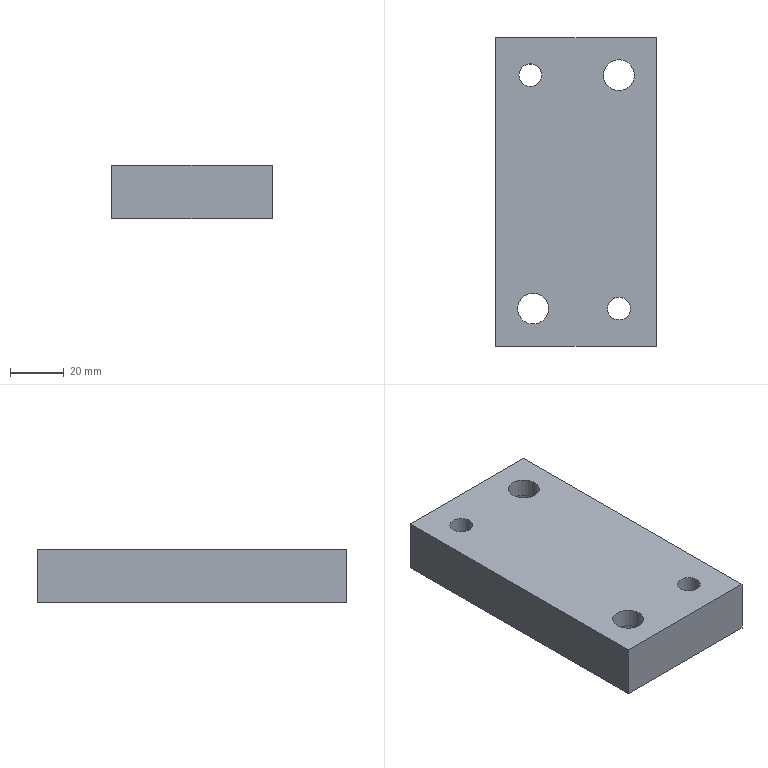Part | STEP file | lll_id610_x_t | 1 solid | 14 faces | box 60 x 115 x 20 mm | volume 127650 mm3 | plane 8 | cylinder 6 | commonest cylinder face diameters 8.505 x2 11.509 x2 18.007 x2
STEP:
#1=CARTESIAN_POINT('',(1834.747,-196.,132.5));
#2=VERTEX_POINT('',#1);
#3=CARTESIAN_POINT('',(1839.,-196.,132.5));
#4=DIRECTION('',(0.,0.,-1.));
#5=DIRECTION('',(-1.,0.,0.));
#6=AXIS2_PLACEMENT_3D('',#3,#4,#5);
#7=CIRCLE('',#6,4.253);
#8=EDGE_CURVE('',#2,#2,#7,.T.);
#9=ORIENTED_EDGE('',*,*,#8,.F.);
#10=EDGE_LOOP('',(#9));
#11=FACE_BOUND('',#10,.T.);
#12=CARTESIAN_POINT('',(1801.747,-109.,132.5));
#13=VERTEX_POINT('',#12);
#14=CARTESIAN_POINT('',(1806.,-109.,132.5));
#15=DIRECTION('',(0.,0.,-1.));
#16=DIRECTION('',(-1.,0.,0.));
#17=AXIS2_PLACEMENT_3D('',#14,#15,#16);
#18=CIRCLE('',#17,4.253);
#19=EDGE_CURVE('',#13,#13,#18,.T.);
#20=ORIENTED_EDGE('',*,*,#19,.F.);
#21=EDGE_LOOP('',(#20));
#22=FACE_BOUND('',#21,.T.);
#23=CARTESIAN_POINT('',(1816.004,-196.,132.5));
#24=VERTEX_POINT('',#23);
#25=CARTESIAN_POINT('',(1807.,-196.,132.5));
#26=DIRECTION('',(0.,0.,1.));
#27=DIRECTION('',(1.,0.,0.));
#28=AXIS2_PLACEMENT_3D('',#25,#26,#27);
#29=CIRCLE('',#28,9.004);
#30=EDGE_CURVE('',#24,#24,#29,.T.);
#31=ORIENTED_EDGE('',*,*,#30,.T.);
#32=EDGE_LOOP('',(#31));
#33=FACE_BOUND('',#32,.T.);
#34=CARTESIAN_POINT('',(1793.,-210.,132.5));
#35=VERTEX_POINT('',#34);
#36=CARTESIAN_POINT('',(1853.,-210.,132.5));
#37=VERTEX_POINT('',#36);
#38=CARTESIAN_POINT('',(1803.,-210.,132.5));
#39=DIRECTION('',(1.,0.,0.));
#40=VECTOR('',#39,1.);
#41=LINE('',#38,#40);
#42=EDGE_CURVE('',#35,#37,#41,.T.);
#43=ORIENTED_EDGE('',*,*,#42,.F.);
#44=CARTESIAN_POINT('',(1793.,-95.,132.5));
#45=VERTEX_POINT('',#44);
#46=CARTESIAN_POINT('',(1793.,-165.,132.5));
#47=DIRECTION('',(0.,1.,0.));
#48=VECTOR('',#47,1.);
#49=LINE('',#46,#48);
#50=EDGE_CURVE('',#35,#45,#49,.T.);
#51=ORIENTED_EDGE('',*,*,#50,.T.);
#52=CARTESIAN_POINT('',(1853.,-95.,132.5));
#53=VERTEX_POINT('',#52);
#54=CARTESIAN_POINT('',(1803.,-95.,132.5));
#55=DIRECTION('',(1.,0.,0.));
#56=VECTOR('',#55,1.);
#57=LINE('',#54,#56);
#58=EDGE_CURVE('',#45,#53,#57,.T.);
#59=ORIENTED_EDGE('',*,*,#58,.T.);
#60=CARTESIAN_POINT('',(1853.,-165.,132.5));
#61=DIRECTION('',(0.,1.,0.));
#62=VECTOR('',#61,1.);
#63=LINE('',#60,#62);
#64=EDGE_CURVE('',#37,#53,#63,.T.);
#65=ORIENTED_EDGE('',*,*,#64,.F.);
#66=EDGE_LOOP('',(#43,#51,#59,#65));
#67=FACE_BOUND('',#66,.T.);
#68=CARTESIAN_POINT('',(1848.004,-109.,132.5));
#69=VERTEX_POINT('',#68);
#70=CARTESIAN_POINT('',(1839.,-109.,132.5));
#71=DIRECTION('',(0.,0.,1.));
#72=DIRECTION('',(1.,0.,0.));
#73=AXIS2_PLACEMENT_3D('',#70,#71,#72);
#74=CIRCLE('',#73,9.004);
#75=EDGE_CURVE('',#69,#69,#74,.T.);
#76=ORIENTED_EDGE('',*,*,#75,.T.);
#77=EDGE_LOOP('',(#76));
#78=FACE_BOUND('',#77,.T.);
#79=CARTESIAN_POINT('',(1803.,-165.,132.5));
#80=DIRECTION('',(0.,0.,-1.));
#81=DIRECTION('',(0.,1.,0.));
#82=AXIS2_PLACEMENT_3D('',#79,#80,#81);
#83=PLANE('',#82);
#84=ADVANCED_FACE('',(#11,#22,#33,#67,#78),#83,.T.);
#85=CARTESIAN_POINT('',(1843.253,-196.,152.5));
#86=VERTEX_POINT('',#85);
#87=CARTESIAN_POINT('',(1839.,-196.,152.5));
#88=DIRECTION('',(0.,0.,1.));
#89=DIRECTION('',(1.,0.,0.));
#90=AXIS2_PLACEMENT_3D('',#87,#88,#89);
#91=CIRCLE('',#90,4.253);
#92=EDGE_CURVE('',#86,#86,#91,.T.);
#93=ORIENTED_EDGE('',*,*,#92,.F.);
#94=EDGE_LOOP('',(#93));
#95=FACE_BOUND('',#94,.T.);
#96=CARTESIAN_POINT('',(1810.253,-109.,152.5));
#97=VERTEX_POINT('',#96);
#98=CARTESIAN_POINT('',(1806.,-109.,152.5));
#99=DIRECTION('',(0.,0.,1.));
#100=DIRECTION('',(1.,0.,0.));
#101=AXIS2_PLACEMENT_3D('',#98,#99,#100);
#102=CIRCLE('',#101,4.253);
#103=EDGE_CURVE('',#97,#97,#102,.T.);
#104=ORIENTED_EDGE('',*,*,#103,.F.);
#105=EDGE_LOOP('',(#104));
#106=FACE_BOUND('',#105,.T.);
#107=CARTESIAN_POINT('',(1844.755,-109.,152.5));
#108=VERTEX_POINT('',#107);
#109=CARTESIAN_POINT('',(1839.,-109.,152.5));
#110=DIRECTION('',(0.,0.,1.));
#111=DIRECTION('',(1.,0.,0.));
#112=AXIS2_PLACEMENT_3D('',#109,#110,#111);
#113=CIRCLE('',#112,5.755);
#114=EDGE_CURVE('',#108,#108,#113,.T.);
#115=ORIENTED_EDGE('',*,*,#114,.F.);
#116=EDGE_LOOP('',(#115));
#117=FACE_BOUND('',#116,.T.);
#118=CARTESIAN_POINT('',(1812.755,-196.,152.5));
#119=VERTEX_POINT('',#118);
#120=CARTESIAN_POINT('',(1807.,-196.,152.5));
#121=DIRECTION('',(0.,0.,1.));
#122=DIRECTION('',(1.,0.,0.));
#123=AXIS2_PLACEMENT_3D('',#120,#121,#122);
#124=CIRCLE('',#123,5.755);
#125=EDGE_CURVE('',#119,#119,#124,.T.);
#126=ORIENTED_EDGE('',*,*,#125,.F.);
#127=EDGE_LOOP('',(#126));
#128=FACE_BOUND('',#127,.T.);
#129=CARTESIAN_POINT('',(1793.,-95.,152.5));
#130=VERTEX_POINT('',#129);
#131=CARTESIAN_POINT('',(1853.,-95.,152.5));
#132=VERTEX_POINT('',#131);
#133=CARTESIAN_POINT('',(1803.,-95.,152.5));
#134=DIRECTION('',(1.,0.,0.));
#135=VECTOR('',#134,1.);
#136=LINE('',#133,#135);
#137=EDGE_CURVE('',#130,#132,#136,.T.);
#138=ORIENTED_EDGE('',*,*,#137,.F.);
#139=CARTESIAN_POINT('',(1793.,-210.,152.5));
#140=VERTEX_POINT('',#139);
#141=CARTESIAN_POINT('',(1793.,-165.,152.5));
#142=DIRECTION('',(0.,-1.,0.));
#143=VECTOR('',#142,1.);
#144=LINE('',#141,#143);
#145=EDGE_CURVE('',#130,#140,#144,.T.);
#146=ORIENTED_EDGE('',*,*,#145,.T.);
#147=CARTESIAN_POINT('',(1853.,-210.,152.5));
#148=VERTEX_POINT('',#147);
#149=CARTESIAN_POINT('',(1803.,-210.,152.5));
#150=DIRECTION('',(1.,0.,0.));
#151=VECTOR('',#150,1.);
#152=LINE('',#149,#151);
#153=EDGE_CURVE('',#140,#148,#152,.T.);
#154=ORIENTED_EDGE('',*,*,#153,.T.);
#155=CARTESIAN_POINT('',(1853.,-165.,152.5));
#156=DIRECTION('',(0.,-1.,0.));
#157=VECTOR('',#156,1.);
#158=LINE('',#155,#157);
#159=EDGE_CURVE('',#132,#148,#158,.T.);
#160=ORIENTED_EDGE('',*,*,#159,.F.);
#161=EDGE_LOOP('',(#138,#146,#154,#160));
#162=FACE_BOUND('',#161,.T.);
#163=CARTESIAN_POINT('',(1803.,-165.,152.5));
#164=DIRECTION('',(0.,0.,1.));
#165=DIRECTION('',(0.,-1.,0.));
#166=AXIS2_PLACEMENT_3D('',#163,#164,#165);
#167=PLANE('',#166);
#168=ADVANCED_FACE('',(#95,#106,#117,#128,#162),#167,.T.);
#169=ORIENTED_EDGE('',*,*,#153,.F.);
#170=CARTESIAN_POINT('',(1793.,-210.,132.5));
#171=DIRECTION('',(0.,0.,1.));
#172=VECTOR('',#171,1.);
#173=LINE('',#170,#172);
#174=EDGE_CURVE('',#35,#140,#173,.T.);
#175=ORIENTED_EDGE('',*,*,#174,.F.);
#176=ORIENTED_EDGE('',*,*,#42,.T.);
#177=CARTESIAN_POINT('',(1853.,-210.,132.5));
#178=DIRECTION('',(0.,0.,1.));
#179=VECTOR('',#178,1.);
#180=LINE('',#177,#179);
#181=EDGE_CURVE('',#37,#148,#180,.T.);
#182=ORIENTED_EDGE('',*,*,#181,.T.);
#183=EDGE_LOOP('',(#169,#175,#176,#182));
#184=FACE_OUTER_BOUND('',#183,.T.);
#185=CARTESIAN_POINT('',(1803.,-210.,132.5));
#186=DIRECTION('',(0.,1.,0.));
#187=DIRECTION('',(0.,0.,1.));
#188=AXIS2_PLACEMENT_3D('',#185,#186,#187);
#189=PLANE('',#188);
#190=ADVANCED_FACE('',(#184),#189,.F.);
#191=CARTESIAN_POINT('',(1793.,-95.,132.5));
#192=DIRECTION('',(0.,0.,1.));
#193=VECTOR('',#192,1.);
#194=LINE('',#191,#193);
#195=EDGE_CURVE('',#45,#130,#194,.T.);
#196=ORIENTED_EDGE('',*,*,#195,.T.);
#197=ORIENTED_EDGE('',*,*,#137,.T.);
#198=CARTESIAN_POINT('',(1853.,-95.,132.5));
#199=DIRECTION('',(0.,0.,1.));
#200=VECTOR('',#199,1.);
#201=LINE('',#198,#200);
#202=EDGE_CURVE('',#53,#132,#201,.T.);
#203=ORIENTED_EDGE('',*,*,#202,.F.);
#204=ORIENTED_EDGE('',*,*,#58,.F.);
#205=EDGE_LOOP('',(#196,#197,#203,#204));
#206=FACE_OUTER_BOUND('',#205,.T.);
#207=CARTESIAN_POINT('',(1803.,-95.,132.5));
#208=DIRECTION('',(0.,1.,0.));
#209=DIRECTION('',(0.,0.,1.));
#210=AXIS2_PLACEMENT_3D('',#207,#208,#209);
#211=PLANE('',#210);
#212=ADVANCED_FACE('',(#206),#211,.T.);
#213=ORIENTED_EDGE('',*,*,#64,.T.);
#214=ORIENTED_EDGE('',*,*,#202,.T.);
#215=ORIENTED_EDGE('',*,*,#159,.T.);
#216=ORIENTED_EDGE('',*,*,#181,.F.);
#217=EDGE_LOOP('',(#213,#214,#215,#216));
#218=FACE_OUTER_BOUND('',#217,.T.);
#219=CARTESIAN_POINT('',(1853.,-165.,132.5));
#220=DIRECTION('',(1.,0.,0.));
#221=DIRECTION('',(0.,0.,-1.));
#222=AXIS2_PLACEMENT_3D('',#219,#220,#221);
#223=PLANE('',#222);
#224=ADVANCED_FACE('',(#218),#223,.T.);
#225=ORIENTED_EDGE('',*,*,#50,.F.);
#226=ORIENTED_EDGE('',*,*,#174,.T.);
#227=ORIENTED_EDGE('',*,*,#145,.F.);
#228=ORIENTED_EDGE('',*,*,#195,.F.);
#229=EDGE_LOOP('',(#225,#226,#227,#228));
#230=FACE_OUTER_BOUND('',#229,.T.);
#231=CARTESIAN_POINT('',(1793.,-165.,132.5));
#232=DIRECTION('',(1.,0.,0.));
#233=DIRECTION('',(0.,0.,-1.));
#234=AXIS2_PLACEMENT_3D('',#231,#232,#233);
#235=PLANE('',#234);
#236=ADVANCED_FACE('',(#230),#235,.F.);
#237=ORIENTED_EDGE('',*,*,#125,.T.);
#238=EDGE_LOOP('',(#237));
#239=FACE_BOUND('',#238,.T.);
#240=CARTESIAN_POINT('',(1812.755,-196.,145.5));
#241=VERTEX_POINT('',#240);
#242=CARTESIAN_POINT('',(1807.,-196.,145.5));
#243=DIRECTION('',(0.,0.,1.));
#244=DIRECTION('',(1.,0.,0.));
#245=AXIS2_PLACEMENT_3D('',#242,#243,#244);
#246=CIRCLE('',#245,5.755);
#247=EDGE_CURVE('',#241,#241,#246,.T.);
#248=ORIENTED_EDGE('',*,*,#247,.F.);
#249=EDGE_LOOP('',(#248));
#250=FACE_BOUND('',#249,.T.);
#251=CARTESIAN_POINT('',(1807.,-196.,127.5));
#252=DIRECTION('',(0.,0.,1.));
#253=DIRECTION('',(1.,0.,0.));
#254=AXIS2_PLACEMENT_3D('',#251,#252,#253);
#255=CYLINDRICAL_SURFACE('',#254,5.755);
#256=ADVANCED_FACE('',(#239,#250),#255,.F.);
#257=ORIENTED_EDGE('',*,*,#247,.T.);
#258=EDGE_LOOP('',(#257));
#259=FACE_BOUND('',#258,.T.);
#260=CARTESIAN_POINT('',(1816.004,-196.,145.5));
#261=VERTEX_POINT('',#260);
#262=CARTESIAN_POINT('',(1807.,-196.,145.5));
#263=DIRECTION('',(0.,0.,1.));
#264=DIRECTION('',(1.,0.,0.));
#265=AXIS2_PLACEMENT_3D('',#262,#263,#264);
#266=CIRCLE('',#265,9.004);
#267=EDGE_CURVE('',#261,#261,#266,.T.);
#268=ORIENTED_EDGE('',*,*,#267,.F.);
#269=EDGE_LOOP('',(#268));
#270=FACE_BOUND('',#269,.T.);
#271=CARTESIAN_POINT('',(1807.,-196.,145.5));
#272=DIRECTION('',(0.,0.,1.));
#273=DIRECTION('',(1.,0.,0.));
#274=AXIS2_PLACEMENT_3D('',#271,#272,#273);
#275=PLANE('',#274);
#276=ADVANCED_FACE('',(#259,#270),#275,.F.);
#277=ORIENTED_EDGE('',*,*,#267,.T.);
#278=EDGE_LOOP('',(#277));
#279=FACE_BOUND('',#278,.T.);
#280=ORIENTED_EDGE('',*,*,#30,.F.);
#281=EDGE_LOOP('',(#280));
#282=FACE_BOUND('',#281,.T.);
#283=CARTESIAN_POINT('',(1807.,-196.,132.5));
#284=DIRECTION('',(0.,0.,1.));
#285=DIRECTION('',(1.,0.,0.));
#286=AXIS2_PLACEMENT_3D('',#283,#284,#285);
#287=CYLINDRICAL_SURFACE('',#286,9.004);
#288=ADVANCED_FACE('',(#279,#282),#287,.F.);
#289=ORIENTED_EDGE('',*,*,#114,.T.);
#290=EDGE_LOOP('',(#289));
#291=FACE_BOUND('',#290,.T.);
#292=CARTESIAN_POINT('',(1844.755,-109.,145.5));
#293=VERTEX_POINT('',#292);
#294=CARTESIAN_POINT('',(1839.,-109.,145.5));
#295=DIRECTION('',(0.,0.,1.));
#296=DIRECTION('',(1.,0.,0.));
#297=AXIS2_PLACEMENT_3D('',#294,#295,#296);
#298=CIRCLE('',#297,5.755);
#299=EDGE_CURVE('',#293,#293,#298,.T.);
#300=ORIENTED_EDGE('',*,*,#299,.F.);
#301=EDGE_LOOP('',(#300));
#302=FACE_BOUND('',#301,.T.);
#303=CARTESIAN_POINT('',(1839.,-109.,127.5));
#304=DIRECTION('',(0.,0.,1.));
#305=DIRECTION('',(1.,0.,0.));
#306=AXIS2_PLACEMENT_3D('',#303,#304,#305);
#307=CYLINDRICAL_SURFACE('',#306,5.755);
#308=ADVANCED_FACE('',(#291,#302),#307,.F.);
#309=ORIENTED_EDGE('',*,*,#299,.T.);
#310=EDGE_LOOP('',(#309));
#311=FACE_BOUND('',#310,.T.);
#312=CARTESIAN_POINT('',(1848.004,-109.,145.5));
#313=VERTEX_POINT('',#312);
#314=CARTESIAN_POINT('',(1839.,-109.,145.5));
#315=DIRECTION('',(0.,0.,1.));
#316=DIRECTION('',(1.,0.,0.));
#317=AXIS2_PLACEMENT_3D('',#314,#315,#316);
#318=CIRCLE('',#317,9.004);
#319=EDGE_CURVE('',#313,#313,#318,.T.);
#320=ORIENTED_EDGE('',*,*,#319,.F.);
#321=EDGE_LOOP('',(#320));
#322=FACE_BOUND('',#321,.T.);
#323=CARTESIAN_POINT('',(1839.,-109.,145.5));
#324=DIRECTION('',(0.,0.,1.));
#325=DIRECTION('',(1.,0.,0.));
#326=AXIS2_PLACEMENT_3D('',#323,#324,#325);
#327=PLANE('',#326);
#328=ADVANCED_FACE('',(#311,#322),#327,.F.);
#329=ORIENTED_EDGE('',*,*,#319,.T.);
#330=EDGE_LOOP('',(#329));
#331=FACE_BOUND('',#330,.T.);
#332=ORIENTED_EDGE('',*,*,#75,.F.);
#333=EDGE_LOOP('',(#332));
#334=FACE_BOUND('',#333,.T.);
#335=CARTESIAN_POINT('',(1839.,-109.,132.5));
#336=DIRECTION('',(0.,0.,1.));
#337=DIRECTION('',(1.,0.,0.));
#338=AXIS2_PLACEMENT_3D('',#335,#336,#337);
#339=CYLINDRICAL_SURFACE('',#338,9.004);
#340=ADVANCED_FACE('',(#331,#334),#339,.F.);
#341=ORIENTED_EDGE('',*,*,#19,.T.);
#342=EDGE_LOOP('',(#341));
#343=FACE_BOUND('',#342,.T.);
#344=ORIENTED_EDGE('',*,*,#103,.T.);
#345=EDGE_LOOP('',(#344));
#346=FACE_BOUND('',#345,.T.);
#347=CARTESIAN_POINT('',(1806.,-109.,127.5));
#348=DIRECTION('',(0.,0.,1.));
#349=DIRECTION('',(1.,0.,0.));
#350=AXIS2_PLACEMENT_3D('',#347,#348,#349);
#351=CYLINDRICAL_SURFACE('',#350,4.253);
#352=ADVANCED_FACE('',(#343,#346),#351,.F.);
#353=ORIENTED_EDGE('',*,*,#8,.T.);
#354=EDGE_LOOP('',(#353));
#355=FACE_BOUND('',#354,.T.);
#356=ORIENTED_EDGE('',*,*,#92,.T.);
#357=EDGE_LOOP('',(#356));
#358=FACE_BOUND('',#357,.T.);
#359=CARTESIAN_POINT('',(1839.,-196.,127.5));
#360=DIRECTION('',(0.,0.,1.));
#361=DIRECTION('',(1.,0.,0.));
#362=AXIS2_PLACEMENT_3D('',#359,#360,#361);
#363=CYLINDRICAL_SURFACE('',#362,4.253);
#364=ADVANCED_FACE('',(#355,#358),#363,.F.);
#365=CLOSED_SHELL('',(#84,#168,#190,#212,#224,#236,#256,#276,#288,#308,#328,#340,#352,#364));
#366=MANIFOLD_SOLID_BREP('',#365);
#367=(LENGTH_UNIT()NAMED_UNIT(*)SI_UNIT(.MILLI.,.METRE.));
#368=UNCERTAINTY_MEASURE_WITH_UNIT(LENGTH_MEASURE(0.00002),#367,'','');
#369=(NAMED_UNIT(*)PLANE_ANGLE_UNIT()SI_UNIT($,.RADIAN.));
#370=PLANE_ANGLE_MEASURE_WITH_UNIT(PLANE_ANGLE_MEASURE(0.01745),#369);
#371=DIMENSIONAL_EXPONENTS(0.,0.,0.,0.,0.,0.,0.);
#372=(CONVERSION_BASED_UNIT('DEGREE',#370)NAMED_UNIT(#371)PLANE_ANGLE_UNIT());
#373=(NAMED_UNIT(*)SI_UNIT($,.STERADIAN.)SOLID_ANGLE_UNIT());
#374=(GEOMETRIC_REPRESENTATION_CONTEXT(3)GLOBAL_UNCERTAINTY_ASSIGNED_CONTEXT((#368))GLOBAL_UNIT_ASSIGNED_CONTEXT((#367,#372,#373))REPRESENTATION_CONTEXT('',''));
#375=ADVANCED_BREP_SHAPE_REPRESENTATION('',(#366),#374);